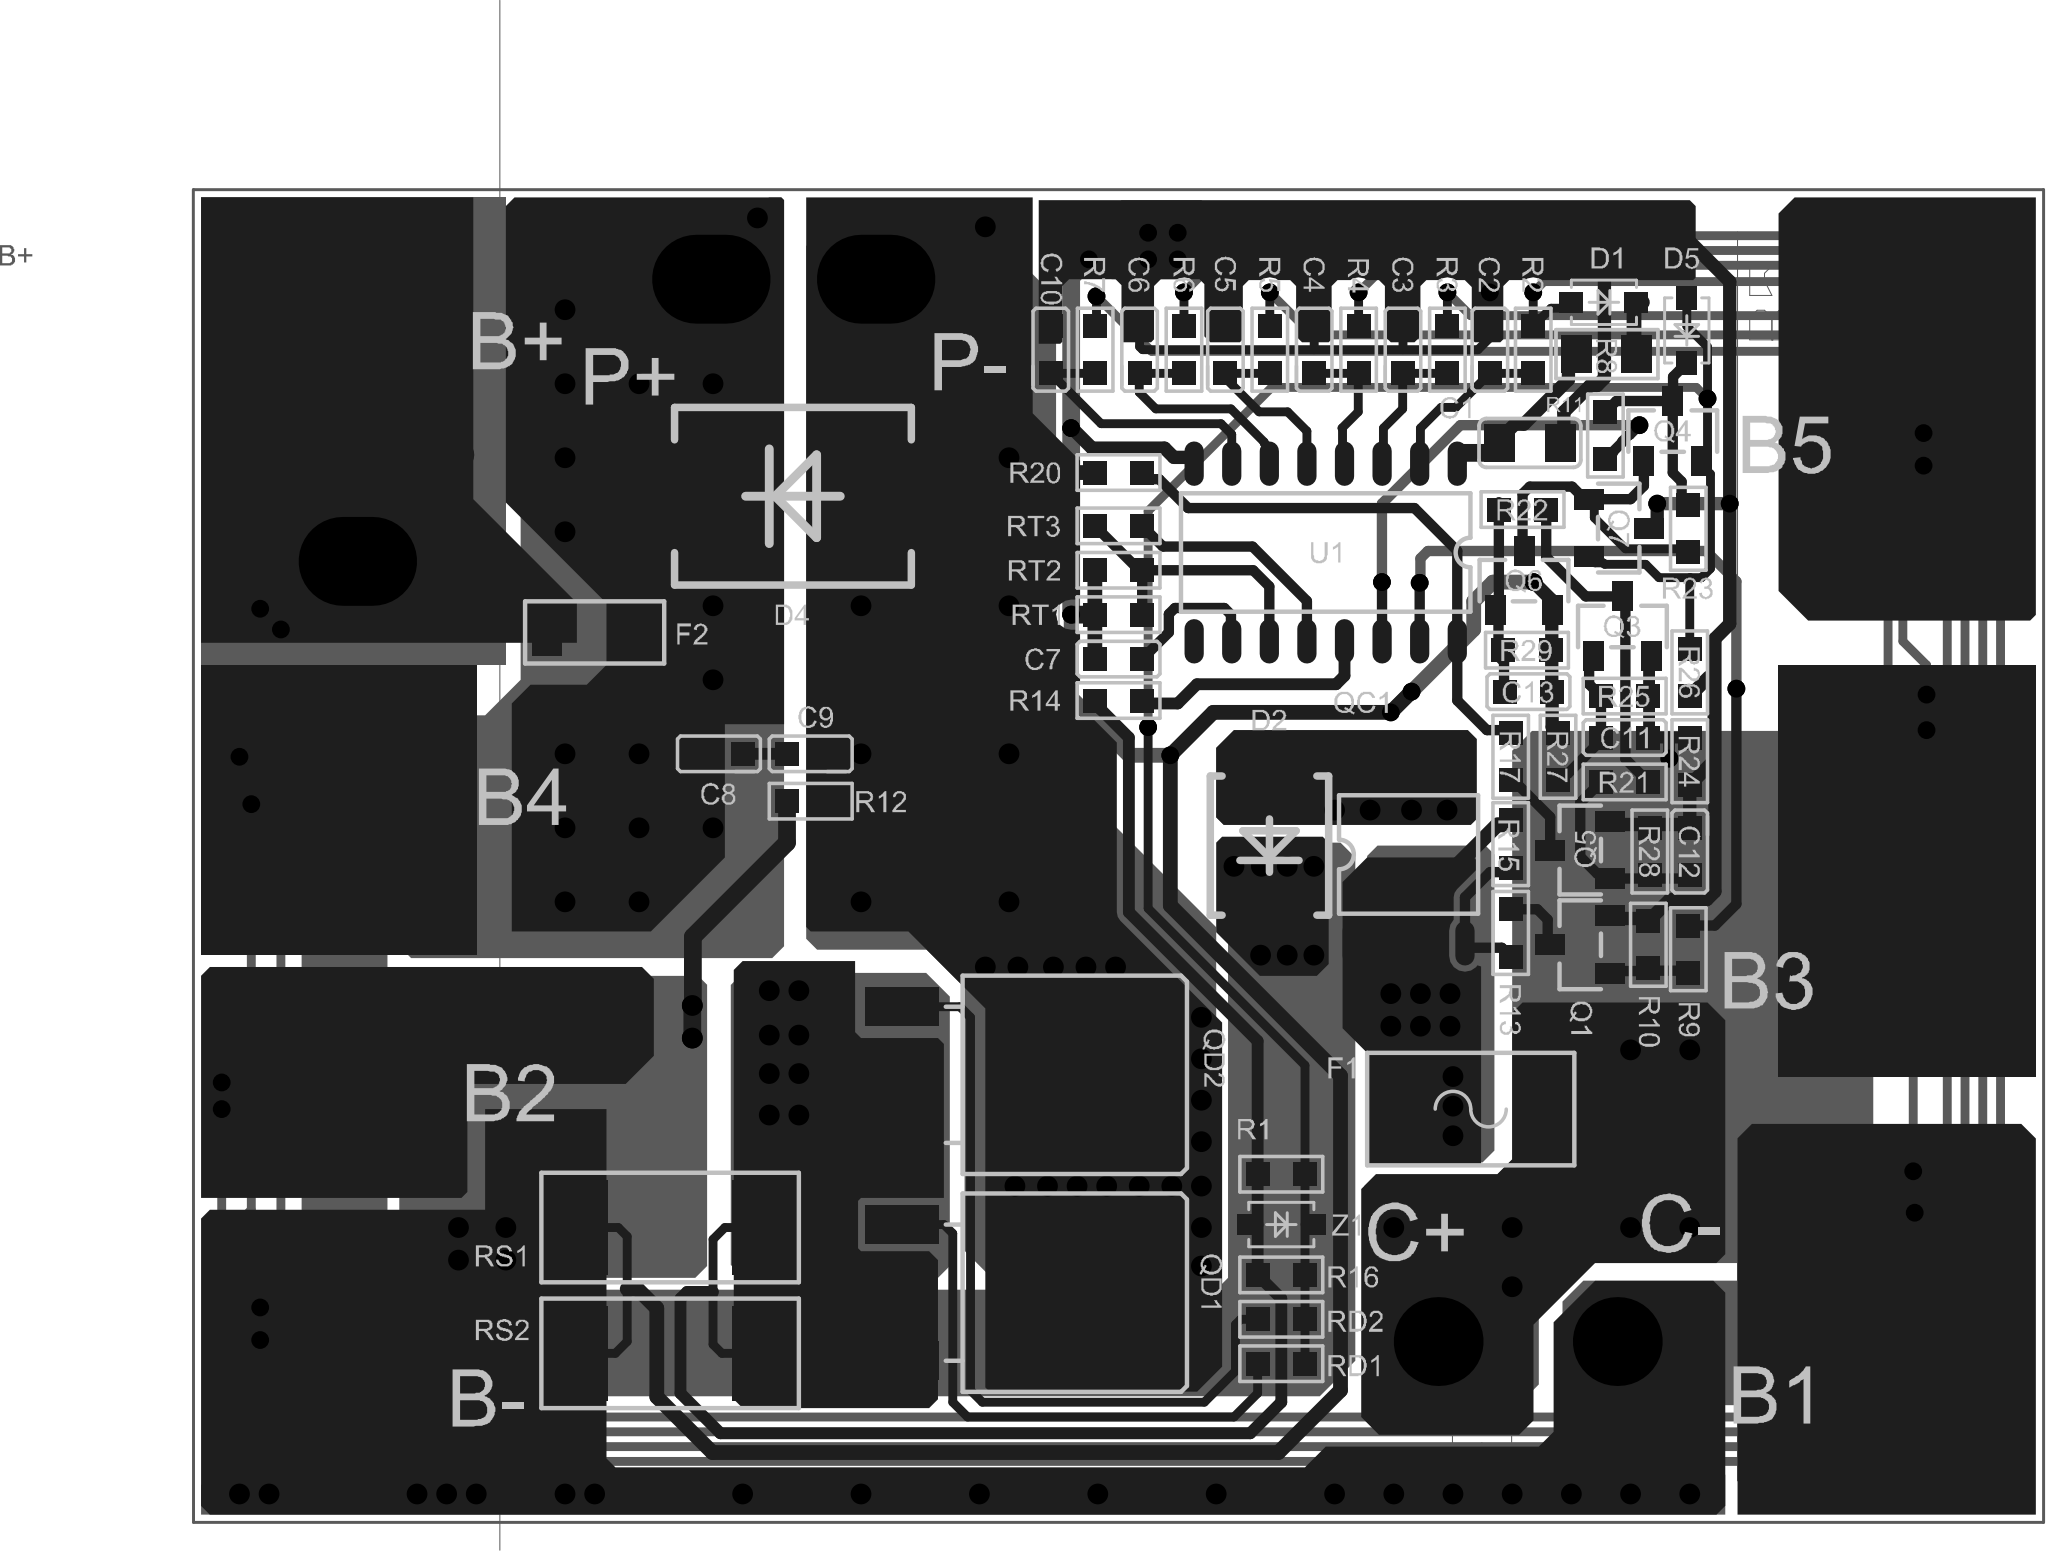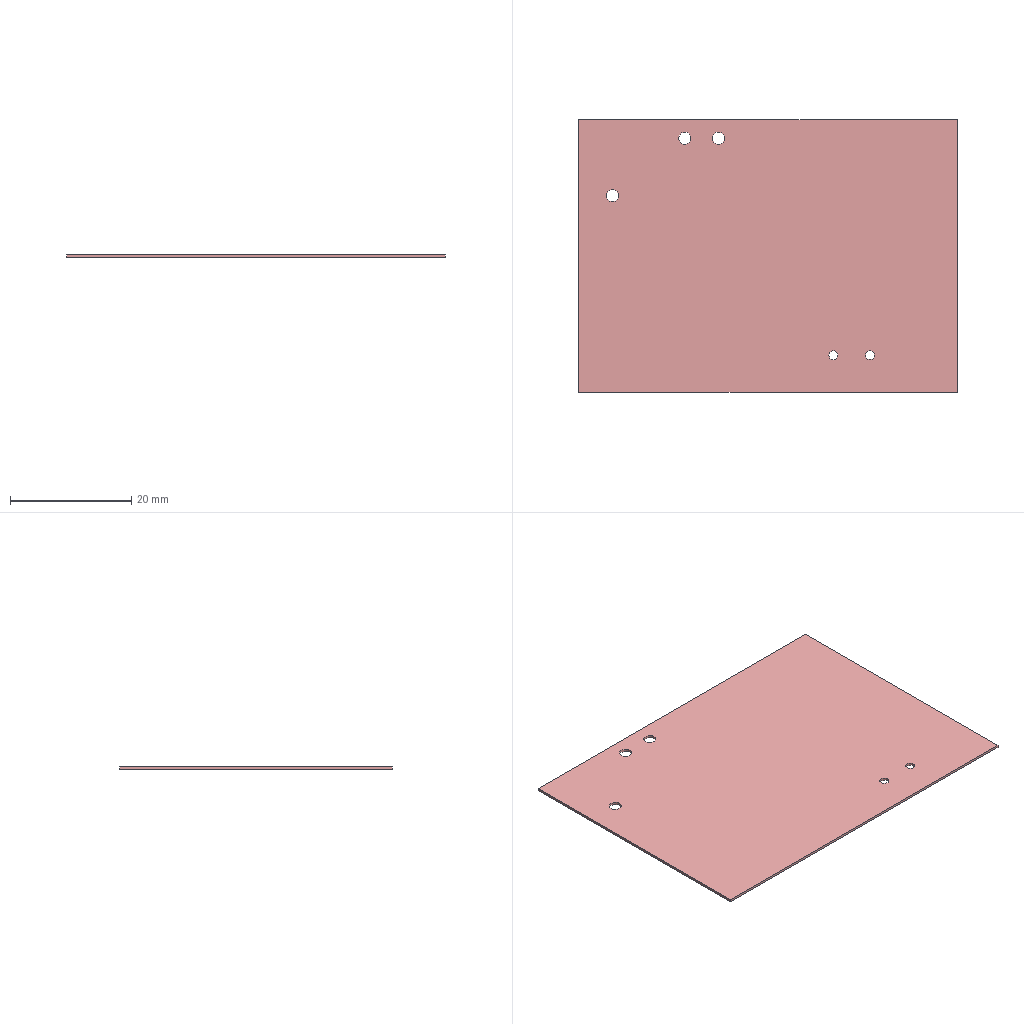Circuit board layout | Altium Designer | box 62.5 x 45 x 0.4 mm
Layer stack:
# Altium Designer layer stack of  (unit mm; dielectric type: 0 none, 1 core, 2 prepreg, 3 surface material)
index,name,kind,layer,copper_thickness_mm,dielectric_type,dielectric_thickness_mm,dielectric_material,dielectric_constant
0,Top Paste,other,,,,,,
1,Top Overlay,other,,,,,,
2,Top Solder,dielectric,,,3,0.0102,Solder Resist,3.5
3,Top Layer,copper,Top Layer,0.0356,,,,
4,Dielectric 1,dielectric,,,0,0.32,FR-4,4.8
5,Bottom Layer,copper,Bottom Layer,0.0356,,,,
6,Bottom Solder,dielectric,,,3,0.0102,Solder Resist,3.5
7,Bottom Overlay,other,,,,,,
8,Bottom Paste,other,,,,,,
# drill layer pairs: low layer,high layer
drill_pair,Top Layer,Bottom Layer
Part placement:
Designator,Comment,Layer,Footprint,Center-X(mm),Center-Y(mm),Rotation
R29,100K,TopLayer,R0603A,112.5,83.5,180
R28,100K,TopLayer,R0603A,116.65,76.7,270
R27,100K,TopLayer,R0603A,113.55,79.9,270
R26,10M,TopLayer,R0603A,118,82.75,90
R25,10K,TopLayer,R0603A,115.8,81.95,0
R24,10K,TopLayer,R0603A,118,79.75,90
R23,1M,TopLayer,R0603A,117.95,87.6,90
R22,1M,TopLayer,R0603A,112.35,88.25,0
R21,1M,TopLayer,R0603A,115.8,79.05,0
R17,0R,TopLayer,R0603A,111.95,79.9,270
Q7,MMBT5401,TopLayer,SOT23-3,115.608,87.625,270
Q6,MMBT5551,TopLayer,SOT23-3,112.4,85.858,0
Q5,MMBT5551,TopLayer,SOT23-3,114.292,76.75,90
Q4,MMBT5551,TopLayer,SOT23-3,117.425,90.908,0
Q3,MMBT5401,TopLayer,SOT23-3,115.725,84.308,0
D5,1N4148SW,TopLayer,SOD323,117.9,94.3,90
C13,NC,TopLayer,C0603A,112.55,82.1,0
C12,NC,TopLayer,C0603A,118,76.7,90
C11,0.1uF,TopLayer,C0603A,115.8,80.55,180
Z1,15V,TopLayer,SOD323,104.2,64.1,180
R1,10M,TopLayer,R0603A,104.2,65.8,0
R12,10M/NC,TopLayer,R0603A,88.3,78.4,0
R4,1K,TopLayer,R0603A,106.811,93.65,270
C10,0.1uF,TopLayer,C0603A,96.411,93.65,270
C1,1uF50V/805,TopLayer,C0805L,112.6,90.5,180
U1,CM10D1*,TopLayer,SOP16L,105.7,86.8,270
D4,RS5M,TopLayer,SMC_A(DO-214AB),87.7,88.7,0
QC1,P MOS*,TopLayer,SOP-8L(T3p),108.5,76.6,90
RT3,1K,TopLayer,R0603A,98.7,87.7,0
RT2,10K B=3435,TopLayer,R0603A,98.7,86.2,0
RT1,10K B=3435,TopLayer,R0603A,98.7,84.7,0
RS2,R010,TopLayer,R2512L,83.55,59.75,0
RS1,R010,TopLayer,R2512L,83.55,64,0
RD2,47R,TopLayer,R0603A,104.2,60.9,0
RD1,47R,TopLayer,R0603A,104.2,59.4,180
R20,1K,TopLayer,R0603A,98.7,89.5,0
R16,10M/NC,TopLayer,R0603A,104.2,62.4,0
R15,3M,TopLayer,R0603A,111.95,76.95,90
R14,1K,TopLayer,R0603A,98.7,81.8,0
R13,3.3M,TopLayer,R0603A,111.95,73.95,270
R11,1K,TopLayer,R0603A,115.15,90.75,270
R10,3.3M,TopLayer,R0603A,116.6,73.55,270
R9,100K,TopLayer,R0603A,117.95,73.4,270
R8,1K/0805,TopLayer,R0805L,115.2,93.5,180
R7,1K,TopLayer,R0603A,97.911,93.65,270
R6,1K,TopLayer,R0603A,100.911,93.65,270
R5,1K,TopLayer,R0603A,103.811,93.65,270
R3,1K,TopLayer,R0603A,109.811,93.65,270
R2,1K,TopLayer,R0603A,112.711,93.65,270
QD2,N MOS*,TopLayer,TO-252,94.612,69.158,270
QD1,N MOS*,TopLayer,TO-252,94.612,61.8,270
Q1,MMBT5551,TopLayer,SOT23-3,114.292,73.55,90
P-,Pth,TopLayer,4*3,90.511,96.03,0
P+,Pth,TopLayer,4*3,84.943,96.03,0
F2,F12F10 32V15A,TopLayer,R1206A,81,84.1,0
F1,PTC,TopLayer,F1812A,110.6,68,0
D2,SS34,TopLayer,SMB(DO-214AA),103.8,76.9,90
D1,BAT46W,TopLayer,SOD323,115.1,95.25,180
C-,Pth,TopLayer,4*3,115.552,60.149,0
C+,Pth,TopLayer,4*3,109.5,60.149,0
C9,0.1uF,TopLayer,C0603A,88.3,80,0
C8,0.1uF,TopLayer,C0603A,85.2,80,0
C7,0.1uF,TopLayer,C0603A,98.7,83.2,180
C6,0.1uF,TopLayer,C0603A,99.411,93.65,270
C5,0.1uF,TopLayer,C0603A,102.311,93.65,270
C4,0.1uF,TopLayer,C0603A,105.311,93.65,270
C3,0.1uF,TopLayer,C0603A,108.311,93.65,270
C2,0.1uF,TopLayer,C0603A,111.246,93.65,270
B-,Pad,TopLayer,Pad10X8mm,72.698,58.039,0
B+,Pad,TopLayer,Pad10X8mm,72.698,95.052,0
B+,Pth,TopLayer,4*3,73,86.5,0
B5,Pad,TopLayer,Pad10X8mm,124.714,95.043,0
B4,Pad,TopLayer,Pad10X8mm,72.698,76.552,0
B3,Pad,TopLayer,Pad10X8mm,124.714,76.535,0
B2,Pad,TopLayer,Pad10X8mm,72.698,68.326,0
B1,Pad,TopLayer,Pad10X8mm,124.7,58.039,0
Pad and via stacks:
# Altium Designer via and pad stacks of  (unit mm). Each distinct definition once, with the count of objects using it.
# via: kind,start_layer,end_layer,hole_mm,diameter_mm,mode(0 simple;1 top-mid-bottom;2 full stack),diameter_per_layer,count,example_net
# pad: kind,layer,hole_mm,hole_type(0 round;1 square;2 slot),plating,top_size,top_shape(1 round;2 rect;3 octagon;9 rounded rect),mid_size,bottom_size,mode,footprint,size_per_layer,count,example
pad,Top Layer,0,0,plated,1.6x3.2,2,1.6x3.2,1.6x3.2,0,F1812A,,2,F1.1
pad,Top Layer,0,0,plated,0.7x1,2,0.7x1,0.7x1,0,SOT23-3,,18,Q4.3
pad,Top Layer,0,0,plated,0.8x0.8,2,0.8x0.8,0.8x0.8,0,R0603A,,62,R26.1
pad,Top Layer,0,0,plated,0.8x0.8,2,0.8x0.8,0.8x0.8,0,C0603A,,24,C11.2
pad,Top Layer,0,0,plated,0.8x0.7,2,0.8x0.7,0.8x0.7,0,SOD323,,6,D5.1
pad,Top Layer,0,2,plated,0.65x1.5,1,0.65x1.5,0.65x1.5,0,SOP16L,,16,U1.5
pad,Top Layer,0,0,plated,1.016x1.27,2,1.016x1.27,1.016x1.27,0,C0805L,,2,C1.1
pad,Top Layer,0,0,plated,2.3x3.2,2,2.3x3.2,2.3x3.2,0,SMC A(DO-214AB),,2,D4.2
pad,Top Layer,0,2,plated,4.2x5.2,2,4.2x5.2,4.2x5.2,0,Pad10X8mm,,7,B+.1
pad,Top Layer,0,0,plated,2x2,1,2x2,2x2,0,,,7,1
pad,Top Layer,0,0,plated,1x1,1,1x1,1x1,0,,,2,1
pad,Top Layer,0,0,plated,1x1.6,2,1x1.6,1x1.6,0,R1206A,,2,F2.1
pad,Top Layer,0,0,plated,6x6,2,6x6,6x6,0,TO-252,,2,QD1.3
pad,Top Layer,0,0,plated,1.3x2.5,2,1.3x2.5,1.3x2.5,0,TO-252,,4,QD1.2
pad,Top Layer,0,0,plated,2x3.2,2,2x3.2,2x3.2,0,R2512L,,4,RS1.2
pad,Top Layer,0,0,plated,2x2.5,2,2x2.5,2x2.5,0,SMB(DO-214AA),,2,D2.2
pad,Top Layer,0,0,plated,1.016x1.27,2,1.016x1.27,1.016x1.27,0,R0805L,,2,R8.2
pad,Top Layer,0,2,plated,0.65x1.5,1,0.65x1.5,0.65x1.5,0,SOP-8L(T3p),,8,QC1.2
pad,Multi-Layer,1.5,0,plated,3x3,1,3x3,3x3,0,4*3,,2,C+.1
pad,Multi-Layer,2,0,plated,4x3,1,4x3,4x3,0,4*3,,3,P-.1
via,Top Layer,Bottom Layer,0.5,0.7,0,,102,NetQD1_2
via,Top Layer,Bottom Layer,0.4,0.6,0,,41,B0
Copper pours:
name,layer,net,type(0 solid;1 hatched;2 none)
Top Layer-C+,Top Layer,C+,0
Top Layer-B5,Top Layer,B5,0
Top Layer-NetC8_1,Top Layer,NetC8_1,0
Top Layer-B0,Top Layer,B0,0
Top Layer-B2,Top Layer,B2,0
Top Layer-NetQD1_2,Top Layer,NetQD1_2,0
B+_L01_P066,Top Layer,B+,0
Top Layer-P-,Top Layer,P-,0
Top Layer-B+ 2,Top Layer,B+,0
Top Layer-B0 2,Top Layer,B0,0
Top Layer-NetD3_2,Top Layer,NetF1_1,0
Top Layer-NetD2_2,Top Layer,NetD2_2,0
Top Layer-B3,Top Layer,B3,0
Top Layer-B1,Top Layer,B1,0
Top Layer-B4,Top Layer,B4,0
Bottom Layer-P-,Bottom Layer,P-,0
NONET_L-01_P-001,Bottom Layer,B0,0
NONET_L-01_P-001,Bottom Layer,B0,0
Bottom Layer-C+,Bottom Layer,C+,0
Top Layer-NetD2_2,Bottom Layer,NetD2_2,0
Bottom Layer-B+,Bottom Layer,B+,0
Bottom Layer-B0,Bottom Layer,B0,0
Bottom Layer-B0 1,Bottom Layer,B0,0
Top Layer-NetD3_2,Bottom Layer,NetF1_1,0
Bottom Layer-NetQD1_2,Bottom Layer,NetQD1_2,0
Bottom Layer-NetC8_1,Bottom Layer,NetC8_1,0
Bottom Layer-B+ 1,Bottom Layer,B+,0
Design rules, without the lines most boards share:
# Altium Designer design rules of  (exported by Altium Designer, unit mm)
# columns: name | kind | enabled | priority | scope1 | scope2 | descriptor | typed fields (field=value)
Schematic Supply Nets_1 | 41 | enabled | 1 | InNet('P-') | All | Supply Net(s)(InNet('P-')) |
Schematic Supply Nets | 41 | enabled | 2 | InNet('B0') | All | Supply Net(s)(InNet('B0')) |
NetAntennae | 56 | enabled | 1 | All | All | Net Antennae (Tolerance=0mm) (All) |
SilkToSilkClearance | 55 | enabled | 1 | All | All | Silk to Silk (Clearance=0mm) (All),(All) |
SilkToSolderMaskClearance | 54 | enabled | 1 | IsPad | All | Silk To Solder Mask (Clearance=0mm) (IsPad),(All) |
MinimumSolderMaskSliver | 53 | enabled | 1 | All | All | Minimum Solder Mask Sliver (Gap=0mm) (All),(All) |
HoleToHoleClearance | 52 | enabled | 1 | All | All | Hole To Hole Clearance (Gap=0mm) (All),(All) | gap=0
DiffPairsRouting | 51 | enabled | 1 | All | All | Differential Pairs Uncoupled Length using the Gap Constraints (Min=0.254mm) (Max=0.254mm) (Prefered=0.254mm)  and Width Constraints (Min=0.381mm) (Max=0.381mm) (Prefered=0.381mm) (All) |
HoleSize | 42 | enabled | 1 | All | All | Hole Size Constraint (Min=0.025mm) (Max=2.54mm) (All) |
Height | 50 | enabled | 1 | All | All | Height Constraint (Min=0mm) (Max=25.4mm) (Prefered=12.7mm) (All) | min_height=0 max_height=25.4
ComponentClearance | 24 | enabled | 1 | All | All | Component Clearance Constraint ( Horizontal Gap = 0mm, Vertical Gap = 0mm ) (All),(All)  | gap=0
SolderMaskExpansion | 13 | enabled | 1 | All | All | Solder Mask Expansion (Expansion =0.102mm) (All) | expansion=0.1016
PasteMaskExpansion | 14 | enabled | 1 | All | All | Paste Mask Expansion (Expansion =0mm) (All) | expansion=0
RoutingVias | 11 | enabled | 1 | All | All | Routing Via (MinHoleWidth=0.4mm) (MaxHoleWidth=0.5mm) (PreferredHoleWidth=0.4mm) (MinWidth=0.6mm) (MaxWidth=0.7mm) (PreferedWidth=0.6mm) (All) | via_min_hole=0.4 via_max_hole=0.5 via_preferred_diameter=0.6 via_preferred_hole=0.4
RoutingCorners | 10 | enabled | 1 | All | All | Routing Corners (Style=45-Degree) (Min Setback=2.54mm) (Max Setback=2.54mm) (All) |
Width | 2 | enabled | 1 | All | All | Width Constraint (Min=0.254mm) (Max=10mm) (Preferred=0.254mm) (All) |
PolygonConnect | 20 | enabled | 1 | All | All | Polygon Connect Rule(Direct Connect )(Conductor Width=0.254mm) (Relief Angle=90 Angle) (Entries=4) (Air Gap Width=0.254mm) (All),(All) | connect_style(0=relief,1=direct,2=none)=1 relief_conductor_width=0.254 relief_entries=4
PlaneClearance | 12 | enabled | 1 | All | All | Power Plane Clearance (Clearance =0.508mm) (All) | clearance=0.508
PlaneConnect | 6 | enabled | 1 | All | All | Power Plane Connect Rule(Direct Connect )(Expansion=0.508mm) (Conductor Width=0.254mm) (Air Gap=0.254mm) (Entries=4) (All) | relief_conductor_width=0.254 relief_entries=4 relief_expansion=0.508
Clearance | 0 | enabled | 1 | All | All | Clearance Constraint (Gap=0.2mm) (All),(All) | gap=0.2